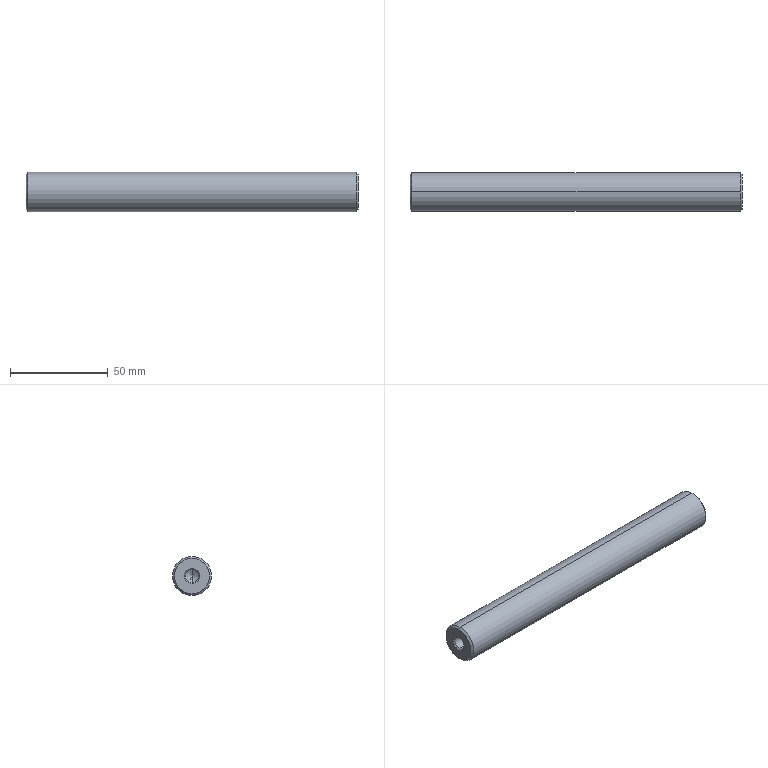Part | STEP file | _PSFJT20-170-M8(0).stp | 1 solid | 14 faces | box 170 x 20 x 20 mm | volume 52553 mm3 | cone 8 | cylinder 4 | plane 2 | commonest cylinder face diameters 6.647 x2 20 x2
STEP:
#1=CARTESIAN_POINT('',(0.,0.,0.));
#2=DIRECTION('',(0.,0.,1.));
#3=DIRECTION('',(1.,0.,0.));
#4=AXIS2_PLACEMENT_3D('',#1,#2,#3);
#5=CARTESIAN_POINT('',(22.081,0.,3.324));
#6=VERTEX_POINT('',#5);
#7=CARTESIAN_POINT('',(22.081,0.,-3.324));
#8=VERTEX_POINT('',#7);
#9=CARTESIAN_POINT('',(22.081,0.,0.));
#10=DIRECTION('',(1.,0.,0.));
#11=DIRECTION('',(0.,0.,-1.));
#12=AXIS2_PLACEMENT_3D('',#9,#10,#11);
#13=CIRCLE('',#12,3.324);
#14=CARTESIAN_POINT('',(23.,0.,0.));
#15=DIRECTION('',(-1.,0.,0.));
#16=DIRECTION('',(0.,0.,1.));
#17=AXIS2_PLACEMENT_3D('',#14,#15,#16);
#18=CONICAL_SURFACE('',#17,1.732,1.047);
#19=CARTESIAN_POINT('',(9.425,0.9188));
#20=DIRECTION('',(-1.,0.));
#21=VECTOR('',#20,1.);
#22=LINE('',#19,#21);
#23=(GEOMETRIC_REPRESENTATION_CONTEXT(2)PARAMETRIC_REPRESENTATION_CONTEXT()REPRESENTATION_CONTEXT('',''));
#24=DEFINITIONAL_REPRESENTATION('',(#22),#23);
#25=PCURVE('',#18,#24);
#26=CARTESIAN_POINT('',(24.,0.,0.));
#27=DIRECTION('',(-1.,0.,0.));
#28=DIRECTION('',(0.,0.,-1.));
#29=AXIS2_PLACEMENT_3D('',#26,#27,#28);
#30=CYLINDRICAL_SURFACE('',#29,3.324);
#31=CARTESIAN_POINT('',(6.283,1.919));
#32=DIRECTION('',(-1.,0.));
#33=VECTOR('',#32,1.);
#34=LINE('',#31,#33);
#35=(GEOMETRIC_REPRESENTATION_CONTEXT(2)PARAMETRIC_REPRESENTATION_CONTEXT()REPRESENTATION_CONTEXT('',''));
#36=DEFINITIONAL_REPRESENTATION('',(#34),#35);
#37=PCURVE('',#30,#36);
#38=SURFACE_CURVE('',#13,(#25,#37),.PCURVE_S1.);
#39=EDGE_CURVE('',#6,#8,#38,.T.);
#40=ORIENTED_EDGE('',*,*,#39,.T.);
#41=CARTESIAN_POINT('',(24.,0.,0.));
#42=VERTEX_POINT('',#41);
#43=CARTESIAN_POINT('',(23.,0.,-1.732));
#44=DIRECTION('',(-0.5,0.,-0.866));
#45=VECTOR('',#44,1.);
#46=LINE('',#43,#45);
#47=CARTESIAN_POINT('',(3.142,0.));
#48=DIRECTION('',(0.,1.));
#49=VECTOR('',#48,1.);
#50=LINE('',#47,#49);
#51=(GEOMETRIC_REPRESENTATION_CONTEXT(2)PARAMETRIC_REPRESENTATION_CONTEXT()REPRESENTATION_CONTEXT('',''));
#52=DEFINITIONAL_REPRESENTATION('',(#50),#51);
#53=PCURVE('',#18,#52);
#54=CARTESIAN_POINT('',(23.,0.,0.));
#55=DIRECTION('',(-1.,0.,0.));
#56=DIRECTION('',(0.,0.,1.));
#57=AXIS2_PLACEMENT_3D('',#54,#55,#56);
#58=CONICAL_SURFACE('',#57,1.732,1.047);
#59=CARTESIAN_POINT('',(3.142,0.));
#60=DIRECTION('',(0.,1.));
#61=VECTOR('',#60,1.);
#62=LINE('',#59,#61);
#63=(GEOMETRIC_REPRESENTATION_CONTEXT(2)PARAMETRIC_REPRESENTATION_CONTEXT()REPRESENTATION_CONTEXT('',''));
#64=DEFINITIONAL_REPRESENTATION('',(#62),#63);
#65=PCURVE('',#58,#64);
#66=SURFACE_CURVE('',#46,(#53,#65),.PCURVE_S1.);
#67=EDGE_CURVE('',#42,#8,#66,.T.);
#68=ORIENTED_EDGE('',*,*,#67,.F.);
#69=CARTESIAN_POINT('',(23.,0.,1.732));
#70=DIRECTION('',(-0.5,0.,0.866));
#71=VECTOR('',#70,1.);
#72=LINE('',#69,#71);
#73=CARTESIAN_POINT('',(6.283,0.));
#74=DIRECTION('',(0.,1.));
#75=VECTOR('',#74,1.);
#76=LINE('',#73,#75);
#77=(GEOMETRIC_REPRESENTATION_CONTEXT(2)PARAMETRIC_REPRESENTATION_CONTEXT()REPRESENTATION_CONTEXT('',''));
#78=DEFINITIONAL_REPRESENTATION('',(#76),#77);
#79=PCURVE('',#18,#78);
#80=CARTESIAN_POINT('',(0.,0.));
#81=DIRECTION('',(0.,1.));
#82=VECTOR('',#81,1.);
#83=LINE('',#80,#82);
#84=(GEOMETRIC_REPRESENTATION_CONTEXT(2)PARAMETRIC_REPRESENTATION_CONTEXT()REPRESENTATION_CONTEXT('',''));
#85=DEFINITIONAL_REPRESENTATION('',(#83),#84);
#86=PCURVE('',#58,#85);
#87=SURFACE_CURVE('',#72,(#79,#86),.PCURVE_S1.);
#88=EDGE_CURVE('',#42,#6,#87,.T.);
#89=ORIENTED_EDGE('',*,*,#88,.T.);
#90=EDGE_LOOP('',(#40,#68,#89));
#91=FACE_BOUND('',#90,.F.);
#92=ADVANCED_FACE('',(#91),#18,.F.);
#93=CARTESIAN_POINT('',(1.,0.,-10.));
#94=VERTEX_POINT('',#93);
#95=CARTESIAN_POINT('',(169.,0.,-10.));
#96=VERTEX_POINT('',#95);
#97=CARTESIAN_POINT('',(1.,0.,-10.));
#98=DIRECTION('',(1.,0.,0.));
#99=VECTOR('',#98,1.);
#100=LINE('',#97,#99);
#101=CARTESIAN_POINT('',(170.,0.,0.));
#102=DIRECTION('',(-1.,0.,0.));
#103=DIRECTION('',(0.,0.,-1.));
#104=AXIS2_PLACEMENT_3D('',#101,#102,#103);
#105=CYLINDRICAL_SURFACE('',#104,10.);
#106=CARTESIAN_POINT('',(0.,169.));
#107=DIRECTION('',(0.,-1.));
#108=VECTOR('',#107,1.);
#109=LINE('',#106,#108);
#110=(GEOMETRIC_REPRESENTATION_CONTEXT(2)PARAMETRIC_REPRESENTATION_CONTEXT()REPRESENTATION_CONTEXT('',''));
#111=DEFINITIONAL_REPRESENTATION('',(#109),#110);
#112=PCURVE('',#105,#111);
#113=CARTESIAN_POINT('',(170.,0.,0.));
#114=DIRECTION('',(-1.,0.,0.));
#115=DIRECTION('',(0.,0.,-1.));
#116=AXIS2_PLACEMENT_3D('',#113,#114,#115);
#117=CYLINDRICAL_SURFACE('',#116,10.);
#118=CARTESIAN_POINT('',(6.283,169.));
#119=DIRECTION('',(0.,-1.));
#120=VECTOR('',#119,1.);
#121=LINE('',#118,#120);
#122=(GEOMETRIC_REPRESENTATION_CONTEXT(2)PARAMETRIC_REPRESENTATION_CONTEXT()REPRESENTATION_CONTEXT('',''));
#123=DEFINITIONAL_REPRESENTATION('',(#121),#122);
#124=PCURVE('',#117,#123);
#125=SURFACE_CURVE('',#100,(#112,#124),.PCURVE_S1.);
#126=EDGE_CURVE('',#94,#96,#125,.T.);
#127=ORIENTED_EDGE('',*,*,#126,.T.);
#128=CARTESIAN_POINT('',(169.,0.,10.));
#129=VERTEX_POINT('',#128);
#130=CARTESIAN_POINT('',(169.,0.,0.));
#131=DIRECTION('',(1.,0.,0.));
#132=DIRECTION('',(0.,0.,-1.));
#133=AXIS2_PLACEMENT_3D('',#130,#131,#132);
#134=CIRCLE('',#133,10.);
#135=CARTESIAN_POINT('',(6.283,1.));
#136=DIRECTION('',(-1.,0.));
#137=VECTOR('',#136,1.);
#138=LINE('',#135,#137);
#139=(GEOMETRIC_REPRESENTATION_CONTEXT(2)PARAMETRIC_REPRESENTATION_CONTEXT()REPRESENTATION_CONTEXT('',''));
#140=DEFINITIONAL_REPRESENTATION('',(#138),#139);
#141=PCURVE('',#105,#140);
#142=CARTESIAN_POINT('',(170.05,0.,0.));
#143=DIRECTION('',(-1.,0.,0.));
#144=DIRECTION('',(0.,0.,1.));
#145=AXIS2_PLACEMENT_3D('',#142,#143,#144);
#146=CONICAL_SURFACE('',#145,8.95,0.7854);
#147=CARTESIAN_POINT('',(9.425,1.05));
#148=DIRECTION('',(-1.,0.));
#149=VECTOR('',#148,1.);
#150=LINE('',#147,#149);
#151=(GEOMETRIC_REPRESENTATION_CONTEXT(2)PARAMETRIC_REPRESENTATION_CONTEXT()REPRESENTATION_CONTEXT('',''));
#152=DEFINITIONAL_REPRESENTATION('',(#150),#151);
#153=PCURVE('',#146,#152);
#154=SURFACE_CURVE('',#134,(#141,#153),.PCURVE_S1.);
#155=EDGE_CURVE('',#129,#96,#154,.T.);
#156=ORIENTED_EDGE('',*,*,#155,.F.);
#157=CARTESIAN_POINT('',(1.,0.,10.));
#158=VERTEX_POINT('',#157);
#159=CARTESIAN_POINT('',(1.,0.,10.));
#160=DIRECTION('',(1.,0.,0.));
#161=VECTOR('',#160,1.);
#162=LINE('',#159,#161);
#163=CARTESIAN_POINT('',(3.142,169.));
#164=DIRECTION('',(0.,-1.));
#165=VECTOR('',#164,1.);
#166=LINE('',#163,#165);
#167=(GEOMETRIC_REPRESENTATION_CONTEXT(2)PARAMETRIC_REPRESENTATION_CONTEXT()REPRESENTATION_CONTEXT('',''));
#168=DEFINITIONAL_REPRESENTATION('',(#166),#167);
#169=PCURVE('',#105,#168);
#170=CARTESIAN_POINT('',(3.142,169.));
#171=DIRECTION('',(0.,-1.));
#172=VECTOR('',#171,1.);
#173=LINE('',#170,#172);
#174=(GEOMETRIC_REPRESENTATION_CONTEXT(2)PARAMETRIC_REPRESENTATION_CONTEXT()REPRESENTATION_CONTEXT('',''));
#175=DEFINITIONAL_REPRESENTATION('',(#173),#174);
#176=PCURVE('',#117,#175);
#177=SURFACE_CURVE('',#162,(#169,#176),.PCURVE_S1.);
#178=EDGE_CURVE('',#158,#129,#177,.T.);
#179=ORIENTED_EDGE('',*,*,#178,.F.);
#180=CARTESIAN_POINT('',(1.,0.,0.));
#181=DIRECTION('',(1.,0.,0.));
#182=DIRECTION('',(0.,0.,-1.));
#183=AXIS2_PLACEMENT_3D('',#180,#181,#182);
#184=CIRCLE('',#183,10.);
#185=CARTESIAN_POINT('',(6.283,169.));
#186=DIRECTION('',(-1.,0.));
#187=VECTOR('',#186,1.);
#188=LINE('',#185,#187);
#189=(GEOMETRIC_REPRESENTATION_CONTEXT(2)PARAMETRIC_REPRESENTATION_CONTEXT()REPRESENTATION_CONTEXT('',''));
#190=DEFINITIONAL_REPRESENTATION('',(#188),#189);
#191=PCURVE('',#105,#190);
#192=CARTESIAN_POINT('',(-0.05,0.,0.));
#193=DIRECTION('',(1.,0.,0.));
#194=DIRECTION('',(0.,0.,-1.));
#195=AXIS2_PLACEMENT_3D('',#192,#193,#194);
#196=CONICAL_SURFACE('',#195,8.95,0.7854);
#197=CARTESIAN_POINT('',(0.,1.05));
#198=DIRECTION('',(1.,0.));
#199=VECTOR('',#198,1.);
#200=LINE('',#197,#199);
#201=(GEOMETRIC_REPRESENTATION_CONTEXT(2)PARAMETRIC_REPRESENTATION_CONTEXT()REPRESENTATION_CONTEXT('',''));
#202=DEFINITIONAL_REPRESENTATION('',(#200),#201);
#203=PCURVE('',#196,#202);
#204=SURFACE_CURVE('',#184,(#191,#203),.PCURVE_S1.);
#205=EDGE_CURVE('',#158,#94,#204,.T.);
#206=ORIENTED_EDGE('',*,*,#205,.T.);
#207=EDGE_LOOP('',(#127,#156,#179,#206));
#208=FACE_BOUND('',#207,.T.);
#209=ADVANCED_FACE('',(#208),#105,.T.);
#210=CARTESIAN_POINT('',(170.,0.,9.));
#211=VERTEX_POINT('',#210);
#212=CARTESIAN_POINT('',(169.,0.,10.));
#213=DIRECTION('',(0.7071,0.,-0.7071));
#214=VECTOR('',#213,1.);
#215=LINE('',#212,#214);
#216=CARTESIAN_POINT('',(170.05,0.,0.));
#217=DIRECTION('',(-1.,0.,0.));
#218=DIRECTION('',(0.,0.,1.));
#219=AXIS2_PLACEMENT_3D('',#216,#217,#218);
#220=CONICAL_SURFACE('',#219,8.95,0.7854);
#221=CARTESIAN_POINT('',(0.,1.05));
#222=DIRECTION('',(0.,-1.));
#223=VECTOR('',#222,1.);
#224=LINE('',#221,#223);
#225=(GEOMETRIC_REPRESENTATION_CONTEXT(2)PARAMETRIC_REPRESENTATION_CONTEXT()REPRESENTATION_CONTEXT('',''));
#226=DEFINITIONAL_REPRESENTATION('',(#224),#225);
#227=PCURVE('',#220,#226);
#228=CARTESIAN_POINT('',(6.283,1.05));
#229=DIRECTION('',(0.,-1.));
#230=VECTOR('',#229,1.);
#231=LINE('',#228,#230);
#232=(GEOMETRIC_REPRESENTATION_CONTEXT(2)PARAMETRIC_REPRESENTATION_CONTEXT()REPRESENTATION_CONTEXT('',''));
#233=DEFINITIONAL_REPRESENTATION('',(#231),#232);
#234=PCURVE('',#146,#233);
#235=SURFACE_CURVE('',#215,(#227,#234),.PCURVE_S1.);
#236=EDGE_CURVE('',#129,#211,#235,.T.);
#237=ORIENTED_EDGE('',*,*,#236,.T.);
#238=CARTESIAN_POINT('',(170.,0.,-9.));
#239=VERTEX_POINT('',#238);
#240=CARTESIAN_POINT('',(170.,0.,0.));
#241=DIRECTION('',(1.,0.,0.));
#242=DIRECTION('',(0.,0.,-1.));
#243=AXIS2_PLACEMENT_3D('',#240,#241,#242);
#244=CIRCLE('',#243,9.);
#245=CARTESIAN_POINT('',(3.142,0.05));
#246=DIRECTION('',(-1.,0.));
#247=VECTOR('',#246,1.);
#248=LINE('',#245,#247);
#249=(GEOMETRIC_REPRESENTATION_CONTEXT(2)PARAMETRIC_REPRESENTATION_CONTEXT()REPRESENTATION_CONTEXT('',''));
#250=DEFINITIONAL_REPRESENTATION('',(#248),#249);
#251=PCURVE('',#220,#250);
#252=CARTESIAN_POINT('',(170.,-9.9,-9.9));
#253=DIRECTION('',(-1.,0.,0.));
#254=DIRECTION('',(0.,0.,1.));
#255=AXIS2_PLACEMENT_3D('',#252,#253,#254);
#256=PLANE('',#255);
#257=CARTESIAN_POINT('',(0.9,9.9));
#258=CARTESIAN_POINT('',(0.9,25.488));
#259=CARTESIAN_POINT('',(14.4,17.694));
#260=CARTESIAN_POINT('',(27.9,9.9));
#261=CARTESIAN_POINT('',(14.4,2.106));
#262=CARTESIAN_POINT('',(0.9,-5.688));
#263=CARTESIAN_POINT('',(0.9,9.9));
#264=(BOUNDED_CURVE()B_SPLINE_CURVE(2,(#257,#258,#259,#260,#261,#262,#263),.UNSPECIFIED.,.T.,.F.)B_SPLINE_CURVE_WITH_KNOTS((1,2,2,2,2,1),(-2.094,0.,2.094,4.189,6.283,8.378),.UNSPECIFIED.)CURVE()GEOMETRIC_REPRESENTATION_ITEM()RATIONAL_B_SPLINE_CURVE((1.,0.5,1.,0.5,1.,0.5,1.))REPRESENTATION_ITEM(''));
#265=(GEOMETRIC_REPRESENTATION_CONTEXT(2)PARAMETRIC_REPRESENTATION_CONTEXT()REPRESENTATION_CONTEXT('',''));
#266=DEFINITIONAL_REPRESENTATION('',(#264),#265);
#267=PCURVE('',#256,#266);
#268=SURFACE_CURVE('',#244,(#251,#267),.PCURVE_S1.);
#269=EDGE_CURVE('',#239,#211,#268,.T.);
#270=ORIENTED_EDGE('',*,*,#269,.F.);
#271=CARTESIAN_POINT('',(169.,0.,-10.));
#272=DIRECTION('',(0.7071,0.,0.7071));
#273=VECTOR('',#272,1.);
#274=LINE('',#271,#273);
#275=CARTESIAN_POINT('',(3.142,1.05));
#276=DIRECTION('',(0.,-1.));
#277=VECTOR('',#276,1.);
#278=LINE('',#275,#277);
#279=(GEOMETRIC_REPRESENTATION_CONTEXT(2)PARAMETRIC_REPRESENTATION_CONTEXT()REPRESENTATION_CONTEXT('',''));
#280=DEFINITIONAL_REPRESENTATION('',(#278),#279);
#281=PCURVE('',#220,#280);
#282=CARTESIAN_POINT('',(3.142,1.05));
#283=DIRECTION('',(0.,-1.));
#284=VECTOR('',#283,1.);
#285=LINE('',#282,#284);
#286=(GEOMETRIC_REPRESENTATION_CONTEXT(2)PARAMETRIC_REPRESENTATION_CONTEXT()REPRESENTATION_CONTEXT('',''));
#287=DEFINITIONAL_REPRESENTATION('',(#285),#286);
#288=PCURVE('',#146,#287);
#289=SURFACE_CURVE('',#274,(#281,#288),.PCURVE_S1.);
#290=EDGE_CURVE('',#96,#239,#289,.T.);
#291=ORIENTED_EDGE('',*,*,#290,.F.);
#292=CARTESIAN_POINT('',(169.,0.,0.));
#293=DIRECTION('',(1.,0.,0.));
#294=DIRECTION('',(0.,0.,-1.));
#295=AXIS2_PLACEMENT_3D('',#292,#293,#294);
#296=CIRCLE('',#295,10.);
#297=CARTESIAN_POINT('',(3.142,1.05));
#298=DIRECTION('',(-1.,0.));
#299=VECTOR('',#298,1.);
#300=LINE('',#297,#299);
#301=(GEOMETRIC_REPRESENTATION_CONTEXT(2)PARAMETRIC_REPRESENTATION_CONTEXT()REPRESENTATION_CONTEXT('',''));
#302=DEFINITIONAL_REPRESENTATION('',(#300),#301);
#303=PCURVE('',#220,#302);
#304=CARTESIAN_POINT('',(6.283,1.));
#305=DIRECTION('',(-1.,0.));
#306=VECTOR('',#305,1.);
#307=LINE('',#304,#306);
#308=(GEOMETRIC_REPRESENTATION_CONTEXT(2)PARAMETRIC_REPRESENTATION_CONTEXT()REPRESENTATION_CONTEXT('',''));
#309=DEFINITIONAL_REPRESENTATION('',(#307),#308);
#310=PCURVE('',#117,#309);
#311=SURFACE_CURVE('',#296,(#303,#310),.PCURVE_S1.);
#312=EDGE_CURVE('',#96,#129,#311,.T.);
#313=ORIENTED_EDGE('',*,*,#312,.T.);
#314=EDGE_LOOP('',(#237,#270,#291,#313));
#315=FACE_BOUND('',#314,.T.);
#316=ADVANCED_FACE('',(#315),#220,.T.);
#317=ORIENTED_EDGE('',*,*,#269,.T.);
#318=CARTESIAN_POINT('',(170.,0.,0.));
#319=DIRECTION('',(1.,0.,0.));
#320=DIRECTION('',(0.,0.,-1.));
#321=AXIS2_PLACEMENT_3D('',#318,#319,#320);
#322=CIRCLE('',#321,9.);
#323=CARTESIAN_POINT('',(0.9,9.9));
#324=CARTESIAN_POINT('',(0.9,25.488));
#325=CARTESIAN_POINT('',(14.4,17.694));
#326=CARTESIAN_POINT('',(27.9,9.9));
#327=CARTESIAN_POINT('',(14.4,2.106));
#328=CARTESIAN_POINT('',(0.9,-5.688));
#329=CARTESIAN_POINT('',(0.9,9.9));
#330=(BOUNDED_CURVE()B_SPLINE_CURVE(2,(#323,#324,#325,#326,#327,#328,#329),.UNSPECIFIED.,.T.,.F.)B_SPLINE_CURVE_WITH_KNOTS((1,2,2,2,2,1),(-2.094,0.,2.094,4.189,6.283,8.378),.UNSPECIFIED.)CURVE()GEOMETRIC_REPRESENTATION_ITEM()RATIONAL_B_SPLINE_CURVE((1.,0.5,1.,0.5,1.,0.5,1.))REPRESENTATION_ITEM(''));
#331=(GEOMETRIC_REPRESENTATION_CONTEXT(2)PARAMETRIC_REPRESENTATION_CONTEXT()REPRESENTATION_CONTEXT('',''));
#332=DEFINITIONAL_REPRESENTATION('',(#330),#331);
#333=PCURVE('',#256,#332);
#334=CARTESIAN_POINT('',(9.425,0.05));
#335=DIRECTION('',(-1.,0.));
#336=VECTOR('',#335,1.);
#337=LINE('',#334,#336);
#338=(GEOMETRIC_REPRESENTATION_CONTEXT(2)PARAMETRIC_REPRESENTATION_CONTEXT()REPRESENTATION_CONTEXT('',''));
#339=DEFINITIONAL_REPRESENTATION('',(#337),#338);
#340=PCURVE('',#146,#339);
#341=SURFACE_CURVE('',#322,(#333,#340),.PCURVE_S1.);
#342=EDGE_CURVE('',#211,#239,#341,.T.);
#343=ORIENTED_EDGE('',*,*,#342,.T.);
#344=EDGE_LOOP('',(#317,#343));
#345=FACE_BOUND('',#344,.T.);
#346=ADVANCED_FACE('',(#345),#256,.F.);
#347=ORIENTED_EDGE('',*,*,#39,.F.);
#348=CARTESIAN_POINT('',(0.6765,0.,3.323));
#349=VERTEX_POINT('',#348);
#350=CARTESIAN_POINT('',(22.081,0.,3.324));
#351=DIRECTION('',(-1.,0.,0.));
#352=VECTOR('',#351,1.);
#353=LINE('',#350,#352);
#354=CARTESIAN_POINT('',(3.142,1.919));
#355=DIRECTION('',(0.,1.));
#356=VECTOR('',#355,1.);
#357=LINE('',#354,#356);
#358=(GEOMETRIC_REPRESENTATION_CONTEXT(2)PARAMETRIC_REPRESENTATION_CONTEXT()REPRESENTATION_CONTEXT('',''));
#359=DEFINITIONAL_REPRESENTATION('',(#357),#358);
#360=PCURVE('',#30,#359);
#361=CARTESIAN_POINT('',(24.,0.,0.));
#362=DIRECTION('',(-1.,0.,0.));
#363=DIRECTION('',(0.,0.,-1.));
#364=AXIS2_PLACEMENT_3D('',#361,#362,#363);
#365=CYLINDRICAL_SURFACE('',#364,3.324);
#366=CARTESIAN_POINT('',(3.142,1.919));
#367=DIRECTION('',(0.,1.));
#368=VECTOR('',#367,1.);
#369=LINE('',#366,#368);
#370=(GEOMETRIC_REPRESENTATION_CONTEXT(2)PARAMETRIC_REPRESENTATION_CONTEXT()REPRESENTATION_CONTEXT('',''));
#371=DEFINITIONAL_REPRESENTATION('',(#369),#370);
#372=PCURVE('',#365,#371);
#373=SURFACE_CURVE('',#353,(#360,#372),.PCURVE_S1.);
#374=EDGE_CURVE('',#6,#349,#373,.T.);
#375=ORIENTED_EDGE('',*,*,#374,.T.);
#376=CARTESIAN_POINT('',(0.6765,0.,-3.324));
#377=VERTEX_POINT('',#376);
#378=CARTESIAN_POINT('',(0.6765,0.,0.));
#379=DIRECTION('',(1.,0.,0.));
#380=DIRECTION('',(0.,0.,-1.));
#381=AXIS2_PLACEMENT_3D('',#378,#379,#380);
#382=CIRCLE('',#381,3.324);
#383=CARTESIAN_POINT('',(6.283,23.323));
#384=DIRECTION('',(-1.,0.));
#385=VECTOR('',#384,1.);
#386=LINE('',#383,#385);
#387=(GEOMETRIC_REPRESENTATION_CONTEXT(2)PARAMETRIC_REPRESENTATION_CONTEXT()REPRESENTATION_CONTEXT('',''));
#388=DEFINITIONAL_REPRESENTATION('',(#386),#387);
#389=PCURVE('',#30,#388);
#390=CARTESIAN_POINT('',(0.7103,0.,0.));
#391=DIRECTION('',(-1.,0.,0.));
#392=DIRECTION('',(0.,0.,1.));
#393=AXIS2_PLACEMENT_3D('',#390,#391,#392);
#394=CONICAL_SURFACE('',#393,3.29,0.7854);
#395=CARTESIAN_POINT('',(9.425,0.03383));
#396=DIRECTION('',(-1.,0.));
#397=VECTOR('',#396,1.);
#398=LINE('',#395,#397);
#399=(GEOMETRIC_REPRESENTATION_CONTEXT(2)PARAMETRIC_REPRESENTATION_CONTEXT()REPRESENTATION_CONTEXT('',''));
#400=DEFINITIONAL_REPRESENTATION('',(#398),#399);
#401=PCURVE('',#394,#400);
#402=SURFACE_CURVE('',#382,(#389,#401),.PCURVE_S1.);
#403=EDGE_CURVE('',#349,#377,#402,.T.);
#404=ORIENTED_EDGE('',*,*,#403,.T.);
#405=CARTESIAN_POINT('',(22.081,0.,-3.324));
#406=DIRECTION('',(-1.,0.,0.));
#407=VECTOR('',#406,1.);
#408=LINE('',#405,#407);
#409=CARTESIAN_POINT('',(0.,1.919));
#410=DIRECTION('',(0.,1.));
#411=VECTOR('',#410,1.);
#412=LINE('',#409,#411);
#413=(GEOMETRIC_REPRESENTATION_CONTEXT(2)PARAMETRIC_REPRESENTATION_CONTEXT()REPRESENTATION_CONTEXT('',''));
#414=DEFINITIONAL_REPRESENTATION('',(#412),#413);
#415=PCURVE('',#30,#414);
#416=CARTESIAN_POINT('',(6.283,1.919));
#417=DIRECTION('',(0.,1.));
#418=VECTOR('',#417,1.);
#419=LINE('',#416,#418);
#420=(GEOMETRIC_REPRESENTATION_CONTEXT(2)PARAMETRIC_REPRESENTATION_CONTEXT()REPRESENTATION_CONTEXT('',''));
#421=DEFINITIONAL_REPRESENTATION('',(#419),#420);
#422=PCURVE('',#365,#421);
#423=SURFACE_CURVE('',#408,(#415,#422),.PCURVE_S1.);
#424=EDGE_CURVE('',#8,#377,#423,.T.);
#425=ORIENTED_EDGE('',*,*,#424,.F.);
#426=EDGE_LOOP('',(#347,#375,#404,#425));
#427=FACE_BOUND('',#426,.F.);
#428=ADVANCED_FACE('',(#427),#30,.F.);
#429=CARTESIAN_POINT('',(0.6765,0.,0.));
#430=DIRECTION('',(1.,0.,0.));
#431=DIRECTION('',(0.,0.,-1.));
#432=AXIS2_PLACEMENT_3D('',#429,#430,#431);
#433=CIRCLE('',#432,3.324);
#434=CARTESIAN_POINT('',(0.7103,0.,0.));
#435=DIRECTION('',(-1.,0.,0.));
#436=DIRECTION('',(0.,0.,1.));
#437=AXIS2_PLACEMENT_3D('',#434,#435,#436);
#438=CONICAL_SURFACE('',#437,3.29,0.7854);
#439=CARTESIAN_POINT('',(3.142,0.03383));
#440=DIRECTION('',(-1.,0.));
#441=VECTOR('',#440,1.);
#442=LINE('',#439,#441);
#443=(GEOMETRIC_REPRESENTATION_CONTEXT(2)PARAMETRIC_REPRESENTATION_CONTEXT()REPRESENTATION_CONTEXT('',''));
#444=DEFINITIONAL_REPRESENTATION('',(#442),#443);
#445=PCURVE('',#438,#444);
#446=CARTESIAN_POINT('',(6.283,23.323));
#447=DIRECTION('',(-1.,0.));
#448=VECTOR('',#447,1.);
#449=LINE('',#446,#448);
#450=(GEOMETRIC_REPRESENTATION_CONTEXT(2)PARAMETRIC_REPRESENTATION_CONTEXT()REPRESENTATION_CONTEXT('',''));
#451=DEFINITIONAL_REPRESENTATION('',(#449),#450);
#452=PCURVE('',#365,#451);
#453=SURFACE_CURVE('',#433,(#445,#452),.PCURVE_S1.);
#454=EDGE_CURVE('',#377,#349,#453,.T.);
#455=ORIENTED_EDGE('',*,*,#454,.F.);
#456=CARTESIAN_POINT('',(0.,0.,-4.));
#457=VERTEX_POINT('',#456);
#458=CARTESIAN_POINT('',(0.6765,0.,-3.324));
#459=DIRECTION('',(-0.7071,0.,-0.7071));
#460=VECTOR('',#459,1.);
#461=LINE('',#458,#460);
#462=CARTESIAN_POINT('',(3.142,0.03383));
#463=DIRECTION('',(0.,1.));
#464=VECTOR('',#463,1.);
#465=LINE('',#462,#464);
#466=(GEOMETRIC_REPRESENTATION_CONTEXT(2)PARAMETRIC_REPRESENTATION_CONTEXT()REPRESENTATION_CONTEXT('',''));
#467=DEFINITIONAL_REPRESENTATION('',(#465),#466);
#468=PCURVE('',#438,#467);
#469=CARTESIAN_POINT('',(3.142,0.03383));
#470=DIRECTION('',(0.,1.));
#471=VECTOR('',#470,1.);
#472=LINE('',#469,#471);
#473=(GEOMETRIC_REPRESENTATION_CONTEXT(2)PARAMETRIC_REPRESENTATION_CONTEXT()REPRESENTATION_CONTEXT('',''));
#474=DEFINITIONAL_REPRESENTATION('',(#472),#473);
#475=PCURVE('',#394,#474);
#476=SURFACE_CURVE('',#461,(#468,#475),.PCURVE_S1.);
#477=EDGE_CURVE('',#377,#457,#476,.T.);
#478=ORIENTED_EDGE('',*,*,#477,.T.);
#479=CARTESIAN_POINT('',(0.,0.,4.));
#480=VERTEX_POINT('',#479);
#481=CARTESIAN_POINT('',(0.,0.,0.));
#482=DIRECTION('',(1.,0.,0.));
#483=DIRECTION('',(0.,0.,-1.));
#484=AXIS2_PLACEMENT_3D('',#481,#482,#483);
#485=CIRCLE('',#484,4.);
#486=CARTESIAN_POINT('',(3.142,0.7103));
#487=DIRECTION('',(-1.,0.));
#488=VECTOR('',#487,1.);
#489=LINE('',#486,#488);
#490=(GEOMETRIC_REPRESENTATION_CONTEXT(2)PARAMETRIC_REPRESENTATION_CONTEXT()REPRESENTATION_CONTEXT('',''));
#491=DEFINITIONAL_REPRESENTATION('',(#489),#490);
#492=PCURVE('',#438,#491);
#493=CARTESIAN_POINT('',(0.,-9.9,9.9));
#494=DIRECTION('',(1.,0.,0.));
#495=DIRECTION('',(0.,1.,0.));
#496=AXIS2_PLACEMENT_3D('',#493,#494,#495);
#497=PLANE('',#496);
#498=CARTESIAN_POINT('',(9.9,-9.9));
#499=DIRECTION('',(0.,-1.));
#500=AXIS2_PLACEMENT_2D('',#498,#499);
#501=CIRCLE('',#500,4.);
#502=(GEOMETRIC_REPRESENTATION_CONTEXT(2)PARAMETRIC_REPRESENTATION_CONTEXT()REPRESENTATION_CONTEXT('',''));
#503=DEFINITIONAL_REPRESENTATION('',(#501),#502);
#504=PCURVE('',#497,#503);
#505=SURFACE_CURVE('',#485,(#492,#504),.PCURVE_S1.);
#506=EDGE_CURVE('',#457,#480,#505,.T.);
#507=ORIENTED_EDGE('',*,*,#506,.T.);
#508=CARTESIAN_POINT('',(0.6765,0.,3.323));
#509=DIRECTION('',(-0.7071,0.,0.7071));
#510=VECTOR('',#509,1.);
#511=LINE('',#508,#510);
#512=CARTESIAN_POINT('',(0.,0.03383));
#513=DIRECTION('',(0.,1.));
#514=VECTOR('',#513,1.);
#515=LINE('',#512,#514);
#516=(GEOMETRIC_REPRESENTATION_CONTEXT(2)PARAMETRIC_REPRESENTATION_CONTEXT()REPRESENTATION_CONTEXT('',''));
#517=DEFINITIONAL_REPRESENTATION('',(#515),#516);
#518=PCURVE('',#438,#517);
#519=CARTESIAN_POINT('',(6.283,0.03383));
#520=DIRECTION('',(0.,1.));
#521=VECTOR('',#520,1.);
#522=LINE('',#519,#521);
#523=(GEOMETRIC_REPRESENTATION_CONTEXT(2)PARAMETRIC_REPRESENTATION_CONTEXT()REPRESENTATION_CONTEXT('',''));
#524=DEFINITIONAL_REPRESENTATION('',(#522),#523);
#525=PCURVE('',#394,#524);
#526=SURFACE_CURVE('',#511,(#518,#525),.PCURVE_S1.);
#527=EDGE_CURVE('',#349,#480,#526,.T.);
#528=ORIENTED_EDGE('',*,*,#527,.F.);
#529=EDGE_LOOP('',(#455,#478,#507,#528));
#530=FACE_BOUND('',#529,.F.);
#531=ADVANCED_FACE('',(#530),#438,.F.);
#532=ORIENTED_EDGE('',*,*,#506,.T.);
#533=CARTESIAN_POINT('',(0.,0.,0.));
#534=DIRECTION('',(1.,0.,0.));
#535=DIRECTION('',(0.,0.,-1.));
#536=AXIS2_PLACEMENT_3D('',#533,#534,#535);
#537=CIRCLE('',#536,4.);
#538=CARTESIAN_POINT('',(9.9,-9.9));
#539=DIRECTION('',(0.,-1.));
#540=AXIS2_PLACEMENT_2D('',#538,#539);
#541=CIRCLE('',#540,4.);
#542=(GEOMETRIC_REPRESENTATION_CONTEXT(2)PARAMETRIC_REPRESENTATION_CONTEXT()REPRESENTATION_CONTEXT('',''));
#543=DEFINITIONAL_REPRESENTATION('',(#541),#542);
#544=PCURVE('',#497,#543);
#545=CARTESIAN_POINT('',(9.425,0.7103));
#546=DIRECTION('',(-1.,0.));
#547=VECTOR('',#546,1.);
#548=LINE('',#545,#547);
#549=(GEOMETRIC_REPRESENTATION_CONTEXT(2)PARAMETRIC_REPRESENTATION_CONTEXT()REPRESENTATION_CONTEXT('',''));
#550=DEFINITIONAL_REPRESENTATION('',(#548),#549);
#551=PCURVE('',#394,#550);
#552=SURFACE_CURVE('',#537,(#544,#551),.PCURVE_S1.);
#553=EDGE_CURVE('',#480,#457,#552,.T.);
#554=ORIENTED_EDGE('',*,*,#553,.T.);
#555=EDGE_LOOP('',(#532,#554));
#556=FACE_BOUND('',#555,.T.);
#557=CARTESIAN_POINT('',(0.,0.,-9.));
#558=VERTEX_POINT('',#557);
#559=CARTESIAN_POINT('',(0.,0.,9.));
#560=VERTEX_POINT('',#559);
#561=CARTESIAN_POINT('',(0.,0.,0.));
#562=DIRECTION('',(1.,0.,0.));
#563=DIRECTION('',(0.,0.,-1.));
#564=AXIS2_PLACEMENT_3D('',#561,#562,#563);
#565=CIRCLE('',#564,9.);
#566=CARTESIAN_POINT('',(9.9,-9.9));
#567=DIRECTION('',(0.,-1.));
#568=AXIS2_PLACEMENT_2D('',#566,#567);
#569=CIRCLE('',#568,9.);
#570=(GEOMETRIC_REPRESENTATION_CONTEXT(2)PARAMETRIC_REPRESENTATION_CONTEXT()REPRESENTATION_CONTEXT('',''));
#571=DEFINITIONAL_REPRESENTATION('',(#569),#570);
#572=PCURVE('',#497,#571);
#573=CARTESIAN_POINT('',(-0.05,0.,0.));
#574=DIRECTION('',(1.,0.,0.));
#575=DIRECTION('',(0.,0.,-1.));
#576=AXIS2_PLACEMENT_3D('',#573,#574,#575);
#577=CONICAL_SURFACE('',#576,8.95,0.7854);
#578=CARTESIAN_POINT('',(0.,0.05));
#579=DIRECTION('',(1.,0.));
#580=VECTOR('',#579,1.);
#581=LINE('',#578,#580);
#582=(GEOMETRIC_REPRESENTATION_CONTEXT(2)PARAMETRIC_REPRESENTATION_CONTEXT()REPRESENTATION_CONTEXT('',''));
#583=DEFINITIONAL_REPRESENTATION('',(#581),#582);
#584=PCURVE('',#577,#583);
#585=SURFACE_CURVE('',#565,(#572,#584),.PCURVE_S1.);
#586=EDGE_CURVE('',#558,#560,#585,.T.);
#587=ORIENTED_EDGE('',*,*,#586,.F.);
#588=CARTESIAN_POINT('',(0.,0.,0.));
#589=DIRECTION('',(1.,0.,0.));
#590=DIRECTION('',(0.,0.,-1.));
#591=AXIS2_PLACEMENT_3D('',#588,#589,#590);
#592=CIRCLE('',#591,9.);
#593=CARTESIAN_POINT('',(9.9,-9.9));
#594=DIRECTION('',(0.,-1.));
#595=AXIS2_PLACEMENT_2D('',#593,#594);
#596=CIRCLE('',#595,9.);
#597=(GEOMETRIC_REPRESENTATION_CONTEXT(2)PARAMETRIC_REPRESENTATION_CONTEXT()REPRESENTATION_CONTEXT('',''));
#598=DEFINITIONAL_REPRESENTATION('',(#596),#597);
#599=PCURVE('',#497,#598);
#600=CARTESIAN_POINT('',(0.,0.05));
#601=DIRECTION('',(1.,0.));
#602=VECTOR('',#601,1.);
#603=LINE('',#600,#602);
#604=(GEOMETRIC_REPRESENTATION_CONTEXT(2)PARAMETRIC_REPRESENTATION_CONTEXT()REPRESENTATION_CONTEXT('',''));
#605=DEFINITIONAL_REPRESENTATION('',(#603),#604);
#606=PCURVE('',#196,#605);
#607=SURFACE_CURVE('',#592,(#599,#606),.PCURVE_S1.);
#608=EDGE_CURVE('',#560,#558,#607,.T.);
#609=ORIENTED_EDGE('',*,*,#608,.F.);
#610=EDGE_LOOP('',(#587,#609));
#611=FACE_BOUND('',#610,.T.);
#612=ADVANCED_FACE('',(#556,#611),#497,.F.);
#613=CARTESIAN_POINT('',(1.,0.,-10.));
#614=DIRECTION('',(-0.7071,0.,0.7071));
#615=VECTOR('',#614,1.);
#616=LINE('',#613,#615);
#617=CARTESIAN_POINT('',(0.,1.05));
#618=DIRECTION('',(0.,-1.));
#619=VECTOR('',#618,1.);
#620=LINE('',#617,#619);
#621=(GEOMETRIC_REPRESENTATION_CONTEXT(2)PARAMETRIC_REPRESENTATION_CONTEXT()REPRESENTATION_CONTEXT('',''));
#622=DEFINITIONAL_REPRESENTATION('',(#620),#621);
#623=PCURVE('',#577,#622);
#624=CARTESIAN_POINT('',(6.283,1.05));
#625=DIRECTION('',(0.,-1.));
#626=VECTOR('',#625,1.);
#627=LINE('',#624,#626);
#628=(GEOMETRIC_REPRESENTATION_CONTEXT(2)PARAMETRIC_REPRESENTATION_CONTEXT()REPRESENTATION_CONTEXT('',''));
#629=DEFINITIONAL_REPRESENTATION('',(#627),#628);
#630=PCURVE('',#196,#629);
#631=SURFACE_CURVE('',#616,(#623,#630),.PCURVE_S1.);
#632=EDGE_CURVE('',#94,#558,#631,.T.);
#633=ORIENTED_EDGE('',*,*,#632,.T.);
#634=ORIENTED_EDGE('',*,*,#586,.T.);
#635=CARTESIAN_POINT('',(1.,0.,10.));
#636=DIRECTION('',(-0.7071,0.,-0.7071));
#637=VECTOR('',#636,1.);
#638=LINE('',#635,#637);
#639=CARTESIAN_POINT('',(3.142,1.05));
#640=DIRECTION('',(0.,-1.));
#641=VECTOR('',#640,1.);
#642=LINE('',#639,#641);
#643=(GEOMETRIC_REPRESENTATION_CONTEXT(2)PARAMETRIC_REPRESENTATION_CONTEXT()REPRESENTATION_CONTEXT('',''));
#644=DEFINITIONAL_REPRESENTATION('',(#642),#643);
#645=PCURVE('',#577,#644);
#646=CARTESIAN_POINT('',(3.142,1.05));
#647=DIRECTION('',(0.,-1.));
#648=VECTOR('',#647,1.);
#649=LINE('',#646,#648);
#650=(GEOMETRIC_REPRESENTATION_CONTEXT(2)PARAMETRIC_REPRESENTATION_CONTEXT()REPRESENTATION_CONTEXT('',''));
#651=DEFINITIONAL_REPRESENTATION('',(#649),#650);
#652=PCURVE('',#196,#651);
#653=SURFACE_CURVE('',#638,(#645,#652),.PCURVE_S1.);
#654=EDGE_CURVE('',#158,#560,#653,.T.);
#655=ORIENTED_EDGE('',*,*,#654,.F.);
#656=CARTESIAN_POINT('',(1.,0.,0.));
#657=DIRECTION('',(1.,0.,0.));
#658=DIRECTION('',(0.,0.,-1.));
#659=AXIS2_PLACEMENT_3D('',#656,#657,#658);
#660=CIRCLE('',#659,10.);
#661=CARTESIAN_POINT('',(0.,1.05));
#662=DIRECTION('',(1.,0.));
#663=VECTOR('',#662,1.);
#664=LINE('',#661,#663);
#665=(GEOMETRIC_REPRESENTATION_CONTEXT(2)PARAMETRIC_REPRESENTATION_CONTEXT()REPRESENTATION_CONTEXT('',''));
#666=DEFINITIONAL_REPRESENTATION('',(#664),#665);
#667=PCURVE('',#577,#666);
#668=CARTESIAN_POINT('',(6.283,169.));
#669=DIRECTION('',(-1.,0.));
#670=VECTOR('',#669,1.);
#671=LINE('',#668,#670);
#672=(GEOMETRIC_REPRESENTATION_CONTEXT(2)PARAMETRIC_REPRESENTATION_CONTEXT()REPRESENTATION_CONTEXT('',''));
#673=DEFINITIONAL_REPRESENTATION('',(#671),#672);
#674=PCURVE('',#117,#673);
#675=SURFACE_CURVE('',#660,(#667,#674),.PCURVE_S1.);
#676=EDGE_CURVE('',#94,#158,#675,.T.);
#677=ORIENTED_EDGE('',*,*,#676,.F.);
#678=EDGE_LOOP('',(#633,#634,#655,#677));
#679=FACE_BOUND('',#678,.T.);
#680=ADVANCED_FACE('',(#679),#577,.T.);
#681=CARTESIAN_POINT('',(22.081,0.,0.));
#682=DIRECTION('',(1.,0.,0.));
#683=DIRECTION('',(0.,0.,-1.));
#684=AXIS2_PLACEMENT_3D('',#681,#682,#683);
#685=CIRCLE('',#684,3.324);
#686=CARTESIAN_POINT('',(3.142,0.9188));
#687=DIRECTION('',(-1.,0.));
#688=VECTOR('',#687,1.);
#689=LINE('',#686,#688);
#690=(GEOMETRIC_REPRESENTATION_CONTEXT(2)PARAMETRIC_REPRESENTATION_CONTEXT()REPRESENTATION_CONTEXT('',''));
#691=DEFINITIONAL_REPRESENTATION('',(#689),#690);
#692=PCURVE('',#58,#691);
#693=CARTESIAN_POINT('',(6.283,1.919));
#694=DIRECTION('',(-1.,0.));
#695=VECTOR('',#694,1.);
#696=LINE('',#693,#695);
#697=(GEOMETRIC_REPRESENTATION_CONTEXT(2)PARAMETRIC_REPRESENTATION_CONTEXT()REPRESENTATION_CONTEXT('',''));
#698=DEFINITIONAL_REPRESENTATION('',(#696),#697);
#699=PCURVE('',#365,#698);
#700=SURFACE_CURVE('',#685,(#692,#699),.PCURVE_S1.);
#701=EDGE_CURVE('',#8,#6,#700,.T.);
#702=ORIENTED_EDGE('',*,*,#701,.T.);
#703=ORIENTED_EDGE('',*,*,#88,.F.);
#704=ORIENTED_EDGE('',*,*,#67,.T.);
#705=EDGE_LOOP('',(#702,#703,#704));
#706=FACE_BOUND('',#705,.F.);
#707=ADVANCED_FACE('',(#706),#58,.F.);
#708=ORIENTED_EDGE('',*,*,#632,.F.);
#709=ORIENTED_EDGE('',*,*,#205,.F.);
#710=ORIENTED_EDGE('',*,*,#654,.T.);
#711=ORIENTED_EDGE('',*,*,#608,.T.);
#712=EDGE_LOOP('',(#708,#709,#710,#711));
#713=FACE_BOUND('',#712,.T.);
#714=ADVANCED_FACE('',(#713),#196,.T.);
#715=ORIENTED_EDGE('',*,*,#553,.T.);
#716=ORIENTED_EDGE('',*,*,#477,.F.);
#717=ORIENTED_EDGE('',*,*,#403,.F.);
#718=ORIENTED_EDGE('',*,*,#527,.T.);
#719=EDGE_LOOP('',(#715,#716,#717,#718));
#720=FACE_BOUND('',#719,.F.);
#721=ADVANCED_FACE('',(#720),#394,.F.);
#722=ORIENTED_EDGE('',*,*,#454,.T.);
#723=ORIENTED_EDGE('',*,*,#374,.F.);
#724=ORIENTED_EDGE('',*,*,#701,.F.);
#725=ORIENTED_EDGE('',*,*,#424,.T.);
#726=EDGE_LOOP('',(#722,#723,#724,#725));
#727=FACE_BOUND('',#726,.F.);
#728=ADVANCED_FACE('',(#727),#365,.F.);
#729=ORIENTED_EDGE('',*,*,#236,.F.);
#730=ORIENTED_EDGE('',*,*,#155,.T.);
#731=ORIENTED_EDGE('',*,*,#290,.T.);
#732=ORIENTED_EDGE('',*,*,#342,.F.);
#733=EDGE_LOOP('',(#729,#730,#731,#732));
#734=FACE_BOUND('',#733,.T.);
#735=ADVANCED_FACE('',(#734),#146,.T.);
#736=ORIENTED_EDGE('',*,*,#126,.F.);
#737=ORIENTED_EDGE('',*,*,#676,.T.);
#738=ORIENTED_EDGE('',*,*,#178,.T.);
#739=ORIENTED_EDGE('',*,*,#312,.F.);
#740=EDGE_LOOP('',(#736,#737,#738,#739));
#741=FACE_BOUND('',#740,.T.);
#742=ADVANCED_FACE('',(#741),#117,.T.);
#743=CLOSED_SHELL('',(#92,#209,#316,#346,#428,#531,#612,#680,#707,#714,#721,#728,#735,#742));
#744=MANIFOLD_SOLID_BREP('',#743);
#745=(LENGTH_UNIT()NAMED_UNIT(*)SI_UNIT(.MILLI.,.METRE.));
#746=UNCERTAINTY_MEASURE_WITH_UNIT(LENGTH_MEASURE(0.0000001),#745,'','');
#747=(NAMED_UNIT(*)PLANE_ANGLE_UNIT()SI_UNIT($,.RADIAN.));
#748=(NAMED_UNIT(*)SI_UNIT($,.STERADIAN.)SOLID_ANGLE_UNIT());
#749=(GEOMETRIC_REPRESENTATION_CONTEXT(3)GLOBAL_UNCERTAINTY_ASSIGNED_CONTEXT((#746))GLOBAL_UNIT_ASSIGNED_CONTEXT((#745,#747,#748))REPRESENTATION_CONTEXT('',''));
#750=ADVANCED_BREP_SHAPE_REPRESENTATION('',(#4,#744),#749);